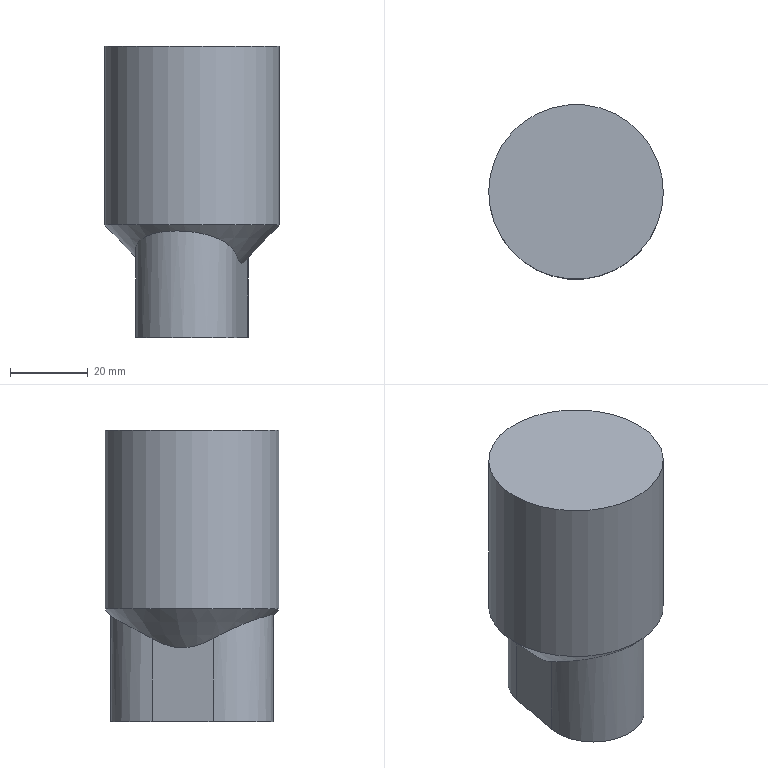Part | NX | features solid 2 | 1 solid | 8 faces | box 45 x 45 x 75 mm | volume 102902 mm3 | plane 4 | cylinder 3 | cone 1 | commonest cylinder face diameters 26.1 x2 45 x1
STEP:
#1=CARTESIAN_POINT('',(-188.837,22.878,56.388));
#2=VERTEX_POINT('',#1);
#3=CARTESIAN_POINT('',(-191.815,7.158,56.388));
#4=VERTEX_POINT('',#3);
#5=CARTESIAN_POINT('',(-188.837,22.878,56.388));
#6=CARTESIAN_POINT('',(-189.067,21.664,55.705));
#7=CARTESIAN_POINT('',(-189.539,19.171,54.515));
#8=CARTESIAN_POINT('',(-190.325,15.023,53.744));
#9=CARTESIAN_POINT('',(-191.11,10.879,54.51));
#10=CARTESIAN_POINT('',(-191.584,8.374,55.704));
#11=CARTESIAN_POINT('',(-191.815,7.158,56.388));
#12=B_SPLINE_CURVE_WITH_KNOTS('',3,(#5,#6,#7,#8,#9,#10,#11),.UNSPECIFIED.,.F.,.F.,(4,1,1,1,4),(0.00000023,0.004199,0.008397,0.0126,0.01679),.UNSPECIFIED.);
#13=EDGE_CURVE('',#2,#4,#12,.T.);
#14=ORIENTED_EDGE('',*,*,#13,.F.);
#15=CARTESIAN_POINT('',(-188.837,22.878,35.));
#16=VERTEX_POINT('',#15);
#17=CARTESIAN_POINT('',(-188.837,22.878,35.));
#18=DIRECTION('',(0.,0.,1.));
#19=VECTOR('',#18,1000.);
#20=LINE('',#17,#19);
#21=EDGE_CURVE('',#16,#2,#20,.T.);
#22=ORIENTED_EDGE('',*,*,#21,.F.);
#23=CARTESIAN_POINT('',(-191.815,7.158,35.));
#24=VERTEX_POINT('',#23);
#25=CARTESIAN_POINT('',(-190.326,15.018,35.));
#26=DIRECTION('',(-0.1861,-0.9825,0.));
#27=VECTOR('',#26,1000.);
#28=LINE('',#25,#27);
#29=EDGE_CURVE('',#16,#24,#28,.T.);
#30=ORIENTED_EDGE('',*,*,#29,.T.);
#31=CARTESIAN_POINT('',(-191.815,7.158,35.));
#32=DIRECTION('',(0.,0.,1.));
#33=VECTOR('',#32,1000.);
#34=LINE('',#31,#33);
#35=EDGE_CURVE('',#24,#4,#34,.T.);
#36=ORIENTED_EDGE('',*,*,#35,.T.);
#37=EDGE_LOOP('',(#14,#22,#30,#36));
#38=FACE_BOUND('',#37,.T.);
#39=CARTESIAN_POINT('',(-190.326,15.018,35.));
#40=DIRECTION('',(-0.9825,0.1861,0.));
#41=DIRECTION('',(0.,0.,1.));
#42=AXIS2_PLACEMENT_3D('',#39,#40,#41);
#43=PLANE('',#42);
#44=ADVANCED_FACE('',(#38),#43,.T.);
#45=ORIENTED_EDGE('',*,*,#29,.F.);
#46=CARTESIAN_POINT('',(-163.193,18.02,35.));
#47=VERTEX_POINT('',#46);
#48=CARTESIAN_POINT('',(-176.015,20.449,35.));
#49=DIRECTION('',(0.,0.,1.));
#50=DIRECTION('',(0.9825,-0.1861,0.));
#51=AXIS2_PLACEMENT_3D('',#48,#49,#50);
#52=CIRCLE('',#51,13.05);
#53=EDGE_CURVE('',#47,#16,#52,.T.);
#54=ORIENTED_EDGE('',*,*,#53,.F.);
#55=CARTESIAN_POINT('',(-166.171,2.3,35.));
#56=VERTEX_POINT('',#55);
#57=CARTESIAN_POINT('',(-164.682,10.16,35.));
#58=DIRECTION('',(0.1861,0.9825,0.));
#59=VECTOR('',#58,1000.);
#60=LINE('',#57,#59);
#61=EDGE_CURVE('',#56,#47,#60,.T.);
#62=ORIENTED_EDGE('',*,*,#61,.F.);
#63=CARTESIAN_POINT('',(-178.993,4.729,35.));
#64=DIRECTION('',(0.,0.,1.));
#65=DIRECTION('',(0.9825,-0.1861,0.));
#66=AXIS2_PLACEMENT_3D('',#63,#64,#65);
#67=CIRCLE('',#66,13.05);
#68=EDGE_CURVE('',#24,#56,#67,.T.);
#69=ORIENTED_EDGE('',*,*,#68,.F.);
#70=EDGE_LOOP('',(#45,#54,#62,#69));
#71=FACE_BOUND('',#70,.T.);
#72=CARTESIAN_POINT('',(-177.504,12.589,35.));
#73=DIRECTION('',(0.,0.,-1.));
#74=DIRECTION('',(-0.9825,0.1861,0.));
#75=AXIS2_PLACEMENT_3D('',#72,#73,#74);
#76=PLANE('',#75);
#77=ADVANCED_FACE('',(#71),#76,.T.);
#78=CARTESIAN_POINT('',(-166.171,2.3,56.388));
#79=VERTEX_POINT('',#78);
#80=CARTESIAN_POINT('',(-163.193,18.02,56.388));
#81=VERTEX_POINT('',#80);
#82=CARTESIAN_POINT('',(-166.171,2.3,56.388));
#83=CARTESIAN_POINT('',(-165.941,3.515,55.705));
#84=CARTESIAN_POINT('',(-165.469,6.007,54.515));
#85=CARTESIAN_POINT('',(-164.683,10.155,53.744));
#86=CARTESIAN_POINT('',(-163.898,14.299,54.51));
#87=CARTESIAN_POINT('',(-163.423,16.804,55.704));
#88=CARTESIAN_POINT('',(-163.193,18.02,56.388));
#89=B_SPLINE_CURVE_WITH_KNOTS('',3,(#82,#83,#84,#85,#86,#87,#88),.UNSPECIFIED.,.F.,.F.,(4,1,1,1,4),(0.00000023,0.004199,0.008397,0.0126,0.01679),.UNSPECIFIED.);
#90=EDGE_CURVE('',#79,#81,#89,.T.);
#91=ORIENTED_EDGE('',*,*,#90,.F.);
#92=CARTESIAN_POINT('',(-166.171,2.3,35.));
#93=DIRECTION('',(0.,0.,1.));
#94=VECTOR('',#93,1000.);
#95=LINE('',#92,#94);
#96=EDGE_CURVE('',#56,#79,#95,.T.);
#97=ORIENTED_EDGE('',*,*,#96,.F.);
#98=ORIENTED_EDGE('',*,*,#61,.T.);
#99=CARTESIAN_POINT('',(-163.193,18.02,35.));
#100=DIRECTION('',(0.,0.,1.));
#101=VECTOR('',#100,1000.);
#102=LINE('',#99,#101);
#103=EDGE_CURVE('',#47,#81,#102,.T.);
#104=ORIENTED_EDGE('',*,*,#103,.T.);
#105=EDGE_LOOP('',(#91,#97,#98,#104));
#106=FACE_BOUND('',#105,.T.);
#107=CARTESIAN_POINT('',(-164.682,10.16,35.));
#108=DIRECTION('',(0.9825,-0.1861,0.));
#109=DIRECTION('',(0.,0.,-1.));
#110=AXIS2_PLACEMENT_3D('',#107,#108,#109);
#111=PLANE('',#110);
#112=ADVANCED_FACE('',(#106),#111,.T.);
#113=CARTESIAN_POINT('',(-188.837,22.878,56.388));
#114=CARTESIAN_POINT('',(-188.251,25.969,58.128));
#115=CARTESIAN_POINT('',(-185.565,30.489,60.419));
#116=CARTESIAN_POINT('',(-179.076,33.517,62.155));
#117=CARTESIAN_POINT('',(-173.544,33.654,62.618));
#118=CARTESIAN_POINT('',(-168.439,31.528,62.165));
#119=CARTESIAN_POINT('',(-164.719,27.651,60.872));
#120=CARTESIAN_POINT('',(-162.867,22.841,58.898));
#121=CARTESIAN_POINT('',(-162.897,19.58,57.266));
#122=CARTESIAN_POINT('',(-163.193,18.02,56.388));
#123=B_SPLINE_CURVE_WITH_KNOTS('',3,(#113,#114,#115,#116,#117,#118,#119,#120,#121,#122),.UNSPECIFIED.,.F.,.F.,(4,1,1,1,1,1,1,4),(0.004699,0.01543,0.02079,0.02615,0.03152,0.03688,0.04224,0.04761),.UNSPECIFIED.);
#124=EDGE_CURVE('',#2,#81,#123,.T.);
#125=ORIENTED_EDGE('',*,*,#124,.F.);
#126=ORIENTED_EDGE('',*,*,#13,.T.);
#127=CARTESIAN_POINT('',(-166.171,2.3,56.388));
#128=CARTESIAN_POINT('',(-166.756,-0.7912,58.128));
#129=CARTESIAN_POINT('',(-169.443,-5.31,60.419));
#130=CARTESIAN_POINT('',(-175.931,-8.339,62.155));
#131=CARTESIAN_POINT('',(-181.463,-8.476,62.618));
#132=CARTESIAN_POINT('',(-186.568,-6.35,62.165));
#133=CARTESIAN_POINT('',(-190.288,-2.473,60.872));
#134=CARTESIAN_POINT('',(-192.14,2.337,58.898));
#135=CARTESIAN_POINT('',(-192.11,5.598,57.266));
#136=CARTESIAN_POINT('',(-191.815,7.158,56.388));
#137=B_SPLINE_CURVE_WITH_KNOTS('',3,(#127,#128,#129,#130,#131,#132,#133,#134,#135,#136),.UNSPECIFIED.,.F.,.F.,(4,1,1,1,1,1,1,4),(0.004699,0.01543,0.02079,0.02615,0.03152,0.03688,0.04224,0.04761),.UNSPECIFIED.);
#138=EDGE_CURVE('',#79,#4,#137,.T.);
#139=ORIENTED_EDGE('',*,*,#138,.F.);
#140=ORIENTED_EDGE('',*,*,#90,.T.);
#141=EDGE_LOOP('',(#125,#126,#139,#140));
#142=FACE_BOUND('',#141,.T.);
#143=CARTESIAN_POINT('',(-155.397,8.401,64.));
#144=VERTEX_POINT('',#143);
#145=CARTESIAN_POINT('',(-177.504,12.589,64.));
#146=DIRECTION('',(0.,0.,1.));
#147=DIRECTION('',(0.9825,-0.1861,0.));
#148=AXIS2_PLACEMENT_3D('',#145,#146,#147);
#149=CIRCLE('',#148,22.5);
#150=EDGE_CURVE('',#144,#144,#149,.T.);
#151=ORIENTED_EDGE('',*,*,#150,.F.);
#152=EDGE_LOOP('',(#151));
#153=FACE_BOUND('',#152,.T.);
#154=CARTESIAN_POINT('',(-177.504,12.589,54.));
#155=DIRECTION('',(0.,0.,1.));
#156=DIRECTION('',(0.9825,-0.1861,0.));
#157=AXIS2_PLACEMENT_3D('',#154,#155,#156);
#158=CONICAL_SURFACE('',#157,13.05,0.7571);
#159=ADVANCED_FACE('',(#142,#153),#158,.T.);
#160=CARTESIAN_POINT('',(-199.611,16.777,110.));
#161=VERTEX_POINT('',#160);
#162=CARTESIAN_POINT('',(-177.504,12.589,110.));
#163=DIRECTION('',(0.,0.,-1.));
#164=DIRECTION('',(-0.9825,0.1861,0.));
#165=AXIS2_PLACEMENT_3D('',#162,#163,#164);
#166=CIRCLE('',#165,22.5);
#167=EDGE_CURVE('',#161,#161,#166,.T.);
#168=ORIENTED_EDGE('',*,*,#167,.F.);
#169=EDGE_LOOP('',(#168));
#170=FACE_BOUND('',#169,.T.);
#171=CARTESIAN_POINT('',(-177.504,12.589,110.));
#172=DIRECTION('',(0.,0.,1.));
#173=DIRECTION('',(0.9825,-0.1861,0.));
#174=AXIS2_PLACEMENT_3D('',#171,#172,#173);
#175=PLANE('',#174);
#176=ADVANCED_FACE('',(#170),#175,.T.);
#177=ORIENTED_EDGE('',*,*,#167,.T.);
#178=EDGE_LOOP('',(#177));
#179=FACE_BOUND('',#178,.T.);
#180=ORIENTED_EDGE('',*,*,#150,.T.);
#181=EDGE_LOOP('',(#180));
#182=FACE_BOUND('',#181,.T.);
#183=CARTESIAN_POINT('',(-177.504,12.589,64.));
#184=DIRECTION('',(0.,0.,1.));
#185=DIRECTION('',(0.9825,-0.1861,0.));
#186=AXIS2_PLACEMENT_3D('',#183,#184,#185);
#187=CYLINDRICAL_SURFACE('',#186,22.5);
#188=ADVANCED_FACE('',(#179,#182),#187,.T.);
#189=ORIENTED_EDGE('',*,*,#35,.F.);
#190=ORIENTED_EDGE('',*,*,#68,.T.);
#191=ORIENTED_EDGE('',*,*,#96,.T.);
#192=ORIENTED_EDGE('',*,*,#138,.T.);
#193=EDGE_LOOP('',(#189,#190,#191,#192));
#194=FACE_BOUND('',#193,.T.);
#195=CARTESIAN_POINT('',(-178.993,4.729,35.));
#196=DIRECTION('',(0.,0.,1.));
#197=DIRECTION('',(0.9825,-0.1861,0.));
#198=AXIS2_PLACEMENT_3D('',#195,#196,#197);
#199=CYLINDRICAL_SURFACE('',#198,13.05);
#200=ADVANCED_FACE('',(#194),#199,.T.);
#201=ORIENTED_EDGE('',*,*,#53,.T.);
#202=ORIENTED_EDGE('',*,*,#21,.T.);
#203=ORIENTED_EDGE('',*,*,#124,.T.);
#204=ORIENTED_EDGE('',*,*,#103,.F.);
#205=EDGE_LOOP('',(#201,#202,#203,#204));
#206=FACE_BOUND('',#205,.T.);
#207=CARTESIAN_POINT('',(-176.015,20.449,35.));
#208=DIRECTION('',(0.,0.,1.));
#209=DIRECTION('',(0.9825,-0.1861,0.));
#210=AXIS2_PLACEMENT_3D('',#207,#208,#209);
#211=CYLINDRICAL_SURFACE('',#210,13.05);
#212=ADVANCED_FACE('',(#206),#211,.T.);
#213=CLOSED_SHELL('',(#44,#77,#112,#159,#176,#188,#200,#212));
#214=MANIFOLD_SOLID_BREP('',#213);
#215=(LENGTH_UNIT()NAMED_UNIT(*)SI_UNIT(.MILLI.,.METRE.));
#216=UNCERTAINTY_MEASURE_WITH_UNIT(LENGTH_MEASURE(0.0508),#215,'','');
#217=(NAMED_UNIT(*)PLANE_ANGLE_UNIT()SI_UNIT($,.RADIAN.));
#218=(NAMED_UNIT(*)SI_UNIT($,.STERADIAN.)SOLID_ANGLE_UNIT());
#219=(GEOMETRIC_REPRESENTATION_CONTEXT(3)GLOBAL_UNCERTAINTY_ASSIGNED_CONTEXT((#216))GLOBAL_UNIT_ASSIGNED_CONTEXT((#215,#217,#218))REPRESENTATION_CONTEXT('',''));
#220=ADVANCED_BREP_SHAPE_REPRESENTATION('',(#214),#219);